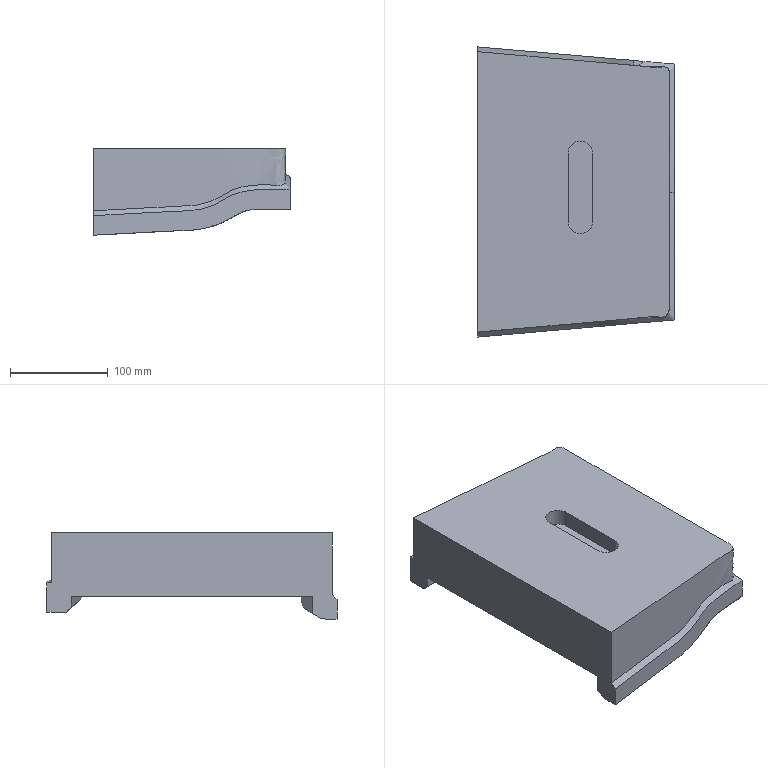Part | NX | features solid 2 | 1 solid | 50 faces | box 201.337 x 297.293 x 88.531 mm | volume 2157323 mm3 | spline 26 | plane 16 | cylinder 8 | commonest cylinder face diameters 30 x6 25 x2